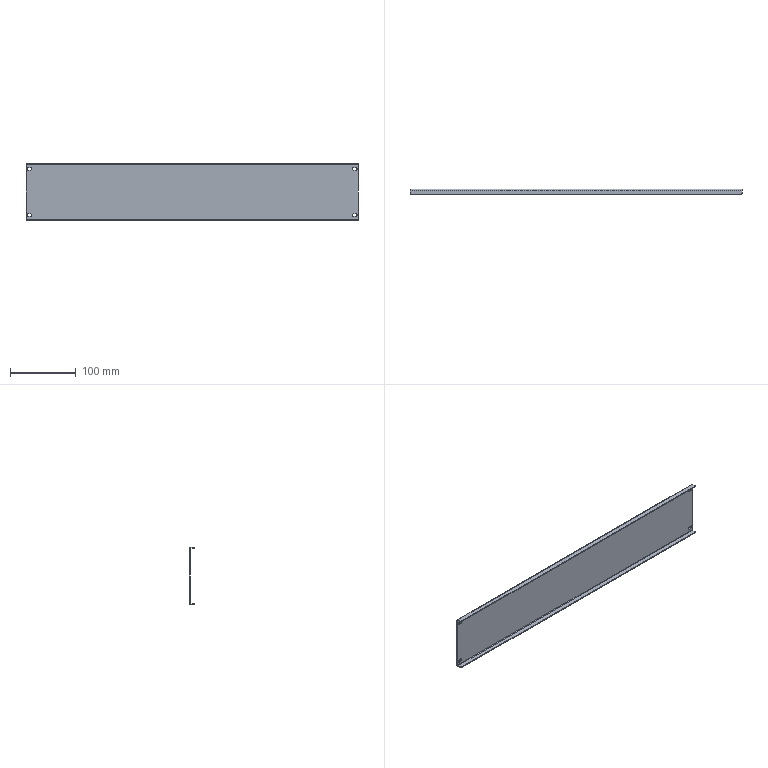Part | STEP file | 1 solid | 42 faces | box 504 x 8.5 x 87 mm | volume 75239 mm3 | plane 26 | cylinder 16 | commonest cylinder face diameters 4 x12 1.473 x2 4.473 x2